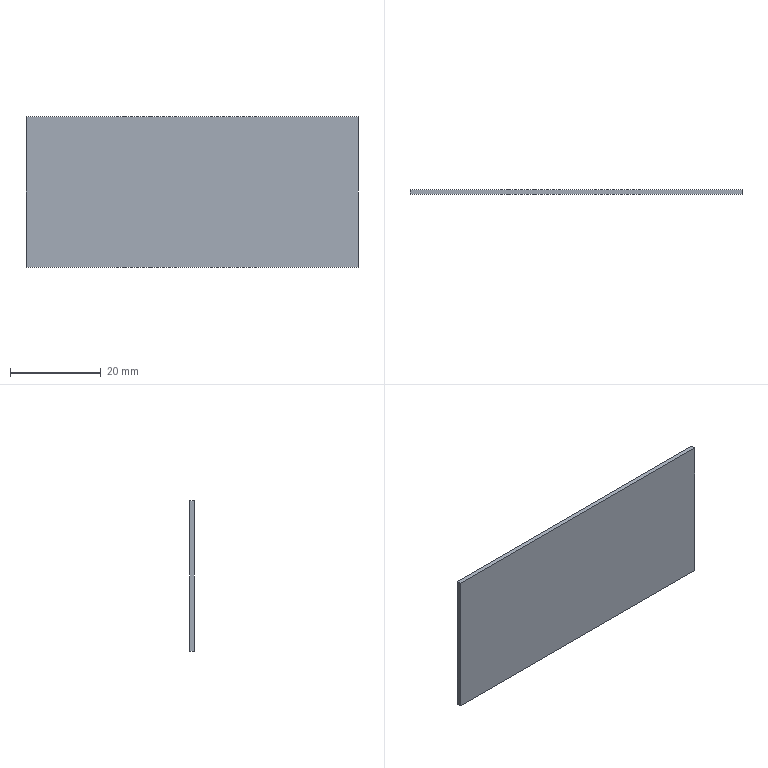Part | STEP file | 09-18 Outlet side seal plate 1 | 1 solid | 6 faces | box 73 x 1 x 33 mm | volume 2409 mm3 | plane 6
STEP:
#1=CARTESIAN_POINT('',(0.,0.,0.));
#2=DIRECTION('',(0.,0.,1.));
#3=DIRECTION('',(1.,0.,0.));
#4=AXIS2_PLACEMENT_3D('',#1,#2,#3);
#5=CARTESIAN_POINT('',(73.,0.,0.));
#6=VERTEX_POINT('',#5);
#7=CARTESIAN_POINT('',(0.,0.,0.));
#8=VERTEX_POINT('',#7);
#9=CARTESIAN_POINT('',(36.5,0.,0.));
#10=DIRECTION('',(-1.,0.,0.));
#11=VECTOR('',#10,1.);
#12=LINE('',#9,#11);
#13=CARTESIAN_POINT('',(73.,0.,0.));
#14=DIRECTION('',(0.,0.,-1.));
#15=DIRECTION('',(-1.,0.,0.));
#16=AXIS2_PLACEMENT_3D('',#13,#14,#15);
#17=PLANE('',#16);
#18=CARTESIAN_POINT('',(36.5,0.));
#19=DIRECTION('',(1.,0.));
#20=VECTOR('',#19,1.);
#21=LINE('',#18,#20);
#22=(GEOMETRIC_REPRESENTATION_CONTEXT(2)PARAMETRIC_REPRESENTATION_CONTEXT()REPRESENTATION_CONTEXT('',''));
#23=DEFINITIONAL_REPRESENTATION('',(#21),#22);
#24=PCURVE('',#17,#23);
#25=CARTESIAN_POINT('',(0.,0.,-33.));
#26=DIRECTION('',(0.,1.,0.));
#27=DIRECTION('',(0.,0.,1.));
#28=AXIS2_PLACEMENT_3D('',#25,#26,#27);
#29=PLANE('',#28);
#30=CARTESIAN_POINT('',(33.,36.5));
#31=DIRECTION('',(0.,-1.));
#32=VECTOR('',#31,1.);
#33=LINE('',#30,#32);
#34=(GEOMETRIC_REPRESENTATION_CONTEXT(2)PARAMETRIC_REPRESENTATION_CONTEXT()REPRESENTATION_CONTEXT('',''));
#35=DEFINITIONAL_REPRESENTATION('',(#33),#34);
#36=PCURVE('',#29,#35);
#37=SURFACE_CURVE('',#12,(#24,#36),.PCURVE_S1.);
#38=EDGE_CURVE('',#6,#8,#37,.T.);
#39=ORIENTED_EDGE('',*,*,#38,.F.);
#40=CARTESIAN_POINT('',(73.,1.,0.));
#41=VERTEX_POINT('',#40);
#42=CARTESIAN_POINT('',(73.,0.5,0.));
#43=DIRECTION('',(0.,1.,0.));
#44=VECTOR('',#43,1.);
#45=LINE('',#42,#44);
#46=CARTESIAN_POINT('',(0.,0.5));
#47=DIRECTION('',(0.,1.));
#48=VECTOR('',#47,1.);
#49=LINE('',#46,#48);
#50=(GEOMETRIC_REPRESENTATION_CONTEXT(2)PARAMETRIC_REPRESENTATION_CONTEXT()REPRESENTATION_CONTEXT('',''));
#51=DEFINITIONAL_REPRESENTATION('',(#49),#50);
#52=PCURVE('',#17,#51);
#53=CARTESIAN_POINT('',(73.,0.,-33.));
#54=DIRECTION('',(-1.,0.,0.));
#55=DIRECTION('',(0.,0.,1.));
#56=AXIS2_PLACEMENT_3D('',#53,#54,#55);
#57=PLANE('',#56);
#58=CARTESIAN_POINT('',(33.,0.5));
#59=DIRECTION('',(0.,1.));
#60=VECTOR('',#59,1.);
#61=LINE('',#58,#60);
#62=(GEOMETRIC_REPRESENTATION_CONTEXT(2)PARAMETRIC_REPRESENTATION_CONTEXT()REPRESENTATION_CONTEXT('',''));
#63=DEFINITIONAL_REPRESENTATION('',(#61),#62);
#64=PCURVE('',#57,#63);
#65=SURFACE_CURVE('',#45,(#52,#64),.PCURVE_S1.);
#66=EDGE_CURVE('',#6,#41,#65,.T.);
#67=ORIENTED_EDGE('',*,*,#66,.T.);
#68=CARTESIAN_POINT('',(0.,1.,0.));
#69=VERTEX_POINT('',#68);
#70=CARTESIAN_POINT('',(36.5,1.,0.));
#71=DIRECTION('',(1.,0.,0.));
#72=VECTOR('',#71,1.);
#73=LINE('',#70,#72);
#74=CARTESIAN_POINT('',(36.5,1.));
#75=DIRECTION('',(-1.,0.));
#76=VECTOR('',#75,1.);
#77=LINE('',#74,#76);
#78=(GEOMETRIC_REPRESENTATION_CONTEXT(2)PARAMETRIC_REPRESENTATION_CONTEXT()REPRESENTATION_CONTEXT('',''));
#79=DEFINITIONAL_REPRESENTATION('',(#77),#78);
#80=PCURVE('',#17,#79);
#81=CARTESIAN_POINT('',(0.,1.,0.));
#82=DIRECTION('',(0.,-1.,0.));
#83=DIRECTION('',(0.,0.,-1.));
#84=AXIS2_PLACEMENT_3D('',#81,#82,#83);
#85=PLANE('',#84);
#86=CARTESIAN_POINT('',(0.,36.5));
#87=DIRECTION('',(0.,1.));
#88=VECTOR('',#87,1.);
#89=LINE('',#86,#88);
#90=(GEOMETRIC_REPRESENTATION_CONTEXT(2)PARAMETRIC_REPRESENTATION_CONTEXT()REPRESENTATION_CONTEXT('',''));
#91=DEFINITIONAL_REPRESENTATION('',(#89),#90);
#92=PCURVE('',#85,#91);
#93=SURFACE_CURVE('',#73,(#80,#92),.PCURVE_S1.);
#94=EDGE_CURVE('',#69,#41,#93,.T.);
#95=ORIENTED_EDGE('',*,*,#94,.F.);
#96=CARTESIAN_POINT('',(0.,0.5,0.));
#97=DIRECTION('',(0.,1.,0.));
#98=VECTOR('',#97,1.);
#99=LINE('',#96,#98);
#100=CARTESIAN_POINT('',(73.,0.5));
#101=DIRECTION('',(0.,1.));
#102=VECTOR('',#101,1.);
#103=LINE('',#100,#102);
#104=(GEOMETRIC_REPRESENTATION_CONTEXT(2)PARAMETRIC_REPRESENTATION_CONTEXT()REPRESENTATION_CONTEXT('',''));
#105=DEFINITIONAL_REPRESENTATION('',(#103),#104);
#106=PCURVE('',#17,#105);
#107=CARTESIAN_POINT('',(0.,0.,-33.));
#108=DIRECTION('',(-1.,0.,0.));
#109=DIRECTION('',(0.,0.,1.));
#110=AXIS2_PLACEMENT_3D('',#107,#108,#109);
#111=PLANE('',#110);
#112=CARTESIAN_POINT('',(33.,0.5));
#113=DIRECTION('',(0.,1.));
#114=VECTOR('',#113,1.);
#115=LINE('',#112,#114);
#116=(GEOMETRIC_REPRESENTATION_CONTEXT(2)PARAMETRIC_REPRESENTATION_CONTEXT()REPRESENTATION_CONTEXT('',''));
#117=DEFINITIONAL_REPRESENTATION('',(#115),#116);
#118=PCURVE('',#111,#117);
#119=SURFACE_CURVE('',#99,(#106,#118),.PCURVE_S1.);
#120=EDGE_CURVE('',#8,#69,#119,.T.);
#121=ORIENTED_EDGE('',*,*,#120,.F.);
#122=EDGE_LOOP('',(#39,#67,#95,#121));
#123=FACE_BOUND('',#122,.T.);
#124=ADVANCED_FACE('',(#123),#17,.F.);
#125=CARTESIAN_POINT('',(73.,0.,-33.));
#126=VERTEX_POINT('',#125);
#127=CARTESIAN_POINT('',(0.,0.,-33.));
#128=VERTEX_POINT('',#127);
#129=CARTESIAN_POINT('',(36.5,0.,-33.));
#130=DIRECTION('',(-1.,0.,0.));
#131=VECTOR('',#130,1.);
#132=LINE('',#129,#131);
#133=CARTESIAN_POINT('',(0.,36.5));
#134=DIRECTION('',(0.,-1.));
#135=VECTOR('',#134,1.);
#136=LINE('',#133,#135);
#137=(GEOMETRIC_REPRESENTATION_CONTEXT(2)PARAMETRIC_REPRESENTATION_CONTEXT()REPRESENTATION_CONTEXT('',''));
#138=DEFINITIONAL_REPRESENTATION('',(#136),#137);
#139=PCURVE('',#29,#138);
#140=CARTESIAN_POINT('',(0.,0.,-33.));
#141=DIRECTION('',(0.,0.,1.));
#142=DIRECTION('',(1.,0.,0.));
#143=AXIS2_PLACEMENT_3D('',#140,#141,#142);
#144=PLANE('',#143);
#145=CARTESIAN_POINT('',(36.5,0.));
#146=DIRECTION('',(-1.,0.));
#147=VECTOR('',#146,1.);
#148=LINE('',#145,#147);
#149=(GEOMETRIC_REPRESENTATION_CONTEXT(2)PARAMETRIC_REPRESENTATION_CONTEXT()REPRESENTATION_CONTEXT('',''));
#150=DEFINITIONAL_REPRESENTATION('',(#148),#149);
#151=PCURVE('',#144,#150);
#152=SURFACE_CURVE('',#132,(#139,#151),.PCURVE_S1.);
#153=EDGE_CURVE('',#126,#128,#152,.T.);
#154=ORIENTED_EDGE('',*,*,#153,.F.);
#155=CARTESIAN_POINT('',(73.,0.,-16.5));
#156=DIRECTION('',(0.,0.,-1.));
#157=VECTOR('',#156,1.);
#158=LINE('',#155,#157);
#159=CARTESIAN_POINT('',(16.5,73.));
#160=DIRECTION('',(-1.,0.));
#161=VECTOR('',#160,1.);
#162=LINE('',#159,#161);
#163=(GEOMETRIC_REPRESENTATION_CONTEXT(2)PARAMETRIC_REPRESENTATION_CONTEXT()REPRESENTATION_CONTEXT('',''));
#164=DEFINITIONAL_REPRESENTATION('',(#162),#163);
#165=PCURVE('',#29,#164);
#166=CARTESIAN_POINT('',(16.5,0.));
#167=DIRECTION('',(-1.,0.));
#168=VECTOR('',#167,1.);
#169=LINE('',#166,#168);
#170=(GEOMETRIC_REPRESENTATION_CONTEXT(2)PARAMETRIC_REPRESENTATION_CONTEXT()REPRESENTATION_CONTEXT('',''));
#171=DEFINITIONAL_REPRESENTATION('',(#169),#170);
#172=PCURVE('',#57,#171);
#173=SURFACE_CURVE('',#158,(#165,#172),.PCURVE_S1.);
#174=EDGE_CURVE('',#6,#126,#173,.T.);
#175=ORIENTED_EDGE('',*,*,#174,.F.);
#176=ORIENTED_EDGE('',*,*,#38,.T.);
#177=CARTESIAN_POINT('',(0.,0.,-16.5));
#178=DIRECTION('',(0.,0.,1.));
#179=VECTOR('',#178,1.);
#180=LINE('',#177,#179);
#181=CARTESIAN_POINT('',(16.5,0.));
#182=DIRECTION('',(1.,0.));
#183=VECTOR('',#182,1.);
#184=LINE('',#181,#183);
#185=(GEOMETRIC_REPRESENTATION_CONTEXT(2)PARAMETRIC_REPRESENTATION_CONTEXT()REPRESENTATION_CONTEXT('',''));
#186=DEFINITIONAL_REPRESENTATION('',(#184),#185);
#187=PCURVE('',#29,#186);
#188=CARTESIAN_POINT('',(16.5,0.));
#189=DIRECTION('',(1.,0.));
#190=VECTOR('',#189,1.);
#191=LINE('',#188,#190);
#192=(GEOMETRIC_REPRESENTATION_CONTEXT(2)PARAMETRIC_REPRESENTATION_CONTEXT()REPRESENTATION_CONTEXT('',''));
#193=DEFINITIONAL_REPRESENTATION('',(#191),#192);
#194=PCURVE('',#111,#193);
#195=SURFACE_CURVE('',#180,(#187,#194),.PCURVE_S1.);
#196=EDGE_CURVE('',#128,#8,#195,.T.);
#197=ORIENTED_EDGE('',*,*,#196,.F.);
#198=EDGE_LOOP('',(#154,#175,#176,#197));
#199=FACE_BOUND('',#198,.T.);
#200=ADVANCED_FACE('',(#199),#29,.F.);
#201=ORIENTED_EDGE('',*,*,#94,.T.);
#202=CARTESIAN_POINT('',(73.,1.,-33.));
#203=VERTEX_POINT('',#202);
#204=CARTESIAN_POINT('',(73.,1.,-16.5));
#205=DIRECTION('',(0.,0.,1.));
#206=VECTOR('',#205,1.);
#207=LINE('',#204,#206);
#208=CARTESIAN_POINT('',(16.5,73.));
#209=DIRECTION('',(-1.,0.));
#210=VECTOR('',#209,1.);
#211=LINE('',#208,#210);
#212=(GEOMETRIC_REPRESENTATION_CONTEXT(2)PARAMETRIC_REPRESENTATION_CONTEXT()REPRESENTATION_CONTEXT('',''));
#213=DEFINITIONAL_REPRESENTATION('',(#211),#212);
#214=PCURVE('',#85,#213);
#215=CARTESIAN_POINT('',(16.5,1.));
#216=DIRECTION('',(1.,0.));
#217=VECTOR('',#216,1.);
#218=LINE('',#215,#217);
#219=(GEOMETRIC_REPRESENTATION_CONTEXT(2)PARAMETRIC_REPRESENTATION_CONTEXT()REPRESENTATION_CONTEXT('',''));
#220=DEFINITIONAL_REPRESENTATION('',(#218),#219);
#221=PCURVE('',#57,#220);
#222=SURFACE_CURVE('',#207,(#214,#221),.PCURVE_S1.);
#223=EDGE_CURVE('',#203,#41,#222,.T.);
#224=ORIENTED_EDGE('',*,*,#223,.F.);
#225=CARTESIAN_POINT('',(0.,1.,-33.));
#226=VERTEX_POINT('',#225);
#227=CARTESIAN_POINT('',(36.5,1.,-33.));
#228=DIRECTION('',(1.,0.,0.));
#229=VECTOR('',#228,1.);
#230=LINE('',#227,#229);
#231=CARTESIAN_POINT('',(33.,36.5));
#232=DIRECTION('',(0.,1.));
#233=VECTOR('',#232,1.);
#234=LINE('',#231,#233);
#235=(GEOMETRIC_REPRESENTATION_CONTEXT(2)PARAMETRIC_REPRESENTATION_CONTEXT()REPRESENTATION_CONTEXT('',''));
#236=DEFINITIONAL_REPRESENTATION('',(#234),#235);
#237=PCURVE('',#85,#236);
#238=CARTESIAN_POINT('',(36.5,1.));
#239=DIRECTION('',(1.,0.));
#240=VECTOR('',#239,1.);
#241=LINE('',#238,#240);
#242=(GEOMETRIC_REPRESENTATION_CONTEXT(2)PARAMETRIC_REPRESENTATION_CONTEXT()REPRESENTATION_CONTEXT('',''));
#243=DEFINITIONAL_REPRESENTATION('',(#241),#242);
#244=PCURVE('',#144,#243);
#245=SURFACE_CURVE('',#230,(#237,#244),.PCURVE_S1.);
#246=EDGE_CURVE('',#226,#203,#245,.T.);
#247=ORIENTED_EDGE('',*,*,#246,.F.);
#248=CARTESIAN_POINT('',(0.,1.,-16.5));
#249=DIRECTION('',(0.,0.,-1.));
#250=VECTOR('',#249,1.);
#251=LINE('',#248,#250);
#252=CARTESIAN_POINT('',(16.5,0.));
#253=DIRECTION('',(1.,0.));
#254=VECTOR('',#253,1.);
#255=LINE('',#252,#254);
#256=(GEOMETRIC_REPRESENTATION_CONTEXT(2)PARAMETRIC_REPRESENTATION_CONTEXT()REPRESENTATION_CONTEXT('',''));
#257=DEFINITIONAL_REPRESENTATION('',(#255),#256);
#258=PCURVE('',#85,#257);
#259=CARTESIAN_POINT('',(16.5,1.));
#260=DIRECTION('',(-1.,0.));
#261=VECTOR('',#260,1.);
#262=LINE('',#259,#261);
#263=(GEOMETRIC_REPRESENTATION_CONTEXT(2)PARAMETRIC_REPRESENTATION_CONTEXT()REPRESENTATION_CONTEXT('',''));
#264=DEFINITIONAL_REPRESENTATION('',(#262),#263);
#265=PCURVE('',#111,#264);
#266=SURFACE_CURVE('',#251,(#258,#265),.PCURVE_S1.);
#267=EDGE_CURVE('',#69,#226,#266,.T.);
#268=ORIENTED_EDGE('',*,*,#267,.F.);
#269=EDGE_LOOP('',(#201,#224,#247,#268));
#270=FACE_BOUND('',#269,.T.);
#271=ADVANCED_FACE('',(#270),#85,.F.);
#272=CARTESIAN_POINT('',(0.,0.5,-33.));
#273=DIRECTION('',(0.,-1.,0.));
#274=VECTOR('',#273,1.);
#275=LINE('',#272,#274);
#276=CARTESIAN_POINT('',(0.,0.5));
#277=DIRECTION('',(0.,-1.));
#278=VECTOR('',#277,1.);
#279=LINE('',#276,#278);
#280=(GEOMETRIC_REPRESENTATION_CONTEXT(2)PARAMETRIC_REPRESENTATION_CONTEXT()REPRESENTATION_CONTEXT('',''));
#281=DEFINITIONAL_REPRESENTATION('',(#279),#280);
#282=PCURVE('',#111,#281);
#283=CARTESIAN_POINT('',(0.,0.5));
#284=DIRECTION('',(0.,-1.));
#285=VECTOR('',#284,1.);
#286=LINE('',#283,#285);
#287=(GEOMETRIC_REPRESENTATION_CONTEXT(2)PARAMETRIC_REPRESENTATION_CONTEXT()REPRESENTATION_CONTEXT('',''));
#288=DEFINITIONAL_REPRESENTATION('',(#286),#287);
#289=PCURVE('',#144,#288);
#290=SURFACE_CURVE('',#275,(#282,#289),.PCURVE_S1.);
#291=EDGE_CURVE('',#226,#128,#290,.T.);
#292=ORIENTED_EDGE('',*,*,#291,.T.);
#293=ORIENTED_EDGE('',*,*,#196,.T.);
#294=ORIENTED_EDGE('',*,*,#120,.T.);
#295=ORIENTED_EDGE('',*,*,#267,.T.);
#296=EDGE_LOOP('',(#292,#293,#294,#295));
#297=FACE_BOUND('',#296,.T.);
#298=ADVANCED_FACE('',(#297),#111,.T.);
#299=ORIENTED_EDGE('',*,*,#246,.T.);
#300=CARTESIAN_POINT('',(73.,0.5,-33.));
#301=DIRECTION('',(0.,1.,0.));
#302=VECTOR('',#301,1.);
#303=LINE('',#300,#302);
#304=CARTESIAN_POINT('',(73.,0.5));
#305=DIRECTION('',(0.,1.));
#306=VECTOR('',#305,1.);
#307=LINE('',#304,#306);
#308=(GEOMETRIC_REPRESENTATION_CONTEXT(2)PARAMETRIC_REPRESENTATION_CONTEXT()REPRESENTATION_CONTEXT('',''));
#309=DEFINITIONAL_REPRESENTATION('',(#307),#308);
#310=PCURVE('',#144,#309);
#311=CARTESIAN_POINT('',(0.,0.5));
#312=DIRECTION('',(0.,1.));
#313=VECTOR('',#312,1.);
#314=LINE('',#311,#313);
#315=(GEOMETRIC_REPRESENTATION_CONTEXT(2)PARAMETRIC_REPRESENTATION_CONTEXT()REPRESENTATION_CONTEXT('',''));
#316=DEFINITIONAL_REPRESENTATION('',(#314),#315);
#317=PCURVE('',#57,#316);
#318=SURFACE_CURVE('',#303,(#310,#317),.PCURVE_S1.);
#319=EDGE_CURVE('',#126,#203,#318,.T.);
#320=ORIENTED_EDGE('',*,*,#319,.F.);
#321=ORIENTED_EDGE('',*,*,#153,.T.);
#322=ORIENTED_EDGE('',*,*,#291,.F.);
#323=EDGE_LOOP('',(#299,#320,#321,#322));
#324=FACE_BOUND('',#323,.T.);
#325=ADVANCED_FACE('',(#324),#144,.F.);
#326=ORIENTED_EDGE('',*,*,#174,.T.);
#327=ORIENTED_EDGE('',*,*,#319,.T.);
#328=ORIENTED_EDGE('',*,*,#223,.T.);
#329=ORIENTED_EDGE('',*,*,#66,.F.);
#330=EDGE_LOOP('',(#326,#327,#328,#329));
#331=FACE_BOUND('',#330,.T.);
#332=ADVANCED_FACE('',(#331),#57,.F.);
#333=CLOSED_SHELL('',(#124,#200,#271,#298,#325,#332));
#334=MANIFOLD_SOLID_BREP('',#333);
#335=(LENGTH_UNIT()NAMED_UNIT(*)SI_UNIT(.MILLI.,.METRE.));
#336=UNCERTAINTY_MEASURE_WITH_UNIT(LENGTH_MEASURE(0.0000001),#335,'','');
#337=(NAMED_UNIT(*)PLANE_ANGLE_UNIT()SI_UNIT($,.RADIAN.));
#338=(NAMED_UNIT(*)SI_UNIT($,.STERADIAN.)SOLID_ANGLE_UNIT());
#339=(GEOMETRIC_REPRESENTATION_CONTEXT(3)GLOBAL_UNCERTAINTY_ASSIGNED_CONTEXT((#336))GLOBAL_UNIT_ASSIGNED_CONTEXT((#335,#337,#338))REPRESENTATION_CONTEXT('',''));
#340=ADVANCED_BREP_SHAPE_REPRESENTATION('',(#4,#334),#339);